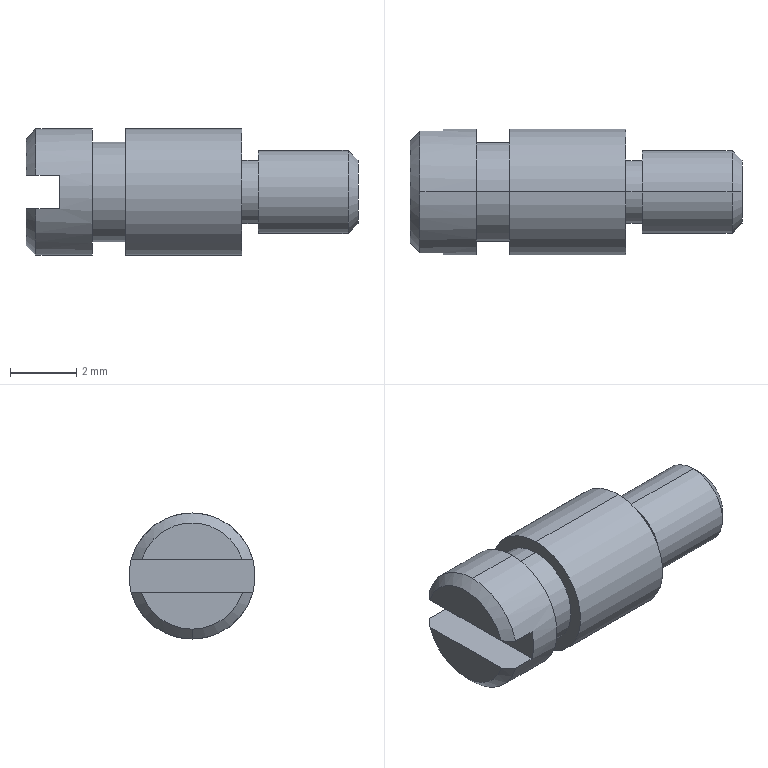Part | SolidWorks | features ICE 1, Revolution 1 | 1 solid | 25 faces | box 10 x 3.8 x 3.8 mm | volume 81.09 mm3 | cylinder 10 | plane 10 | cone 5 | commonest cylinder face diameters 3.8 x4 1.9 x2 2.5 x2 3 x2
STEP:
#1=CARTESIAN_POINT('',(0.,0.,0.95));
#2=VERTEX_POINT('',#1);
#3=CARTESIAN_POINT('',(0.,0.,-0.95));
#4=VERTEX_POINT('',#3);
#5=CARTESIAN_POINT('',(0.,0.,0.));
#6=DIRECTION('',(-1.,0.,0.));
#7=DIRECTION('',(0.,0.,1.));
#8=AXIS2_PLACEMENT_3D('',#5,#6,#7);
#9=CIRCLE('',#8,0.95);
#10=EDGE_CURVE('',#2,#4,#9,.T.);
#11=ORIENTED_EDGE('',*,*,#10,.T.);
#12=CARTESIAN_POINT('',(-0.3,0.,-1.25));
#13=VERTEX_POINT('',#12);
#14=CARTESIAN_POINT('',(0.,0.,-0.95));
#15=DIRECTION('',(-0.7071,0.,-0.7071));
#16=VECTOR('',#15,1000.);
#17=LINE('',#14,#16);
#18=EDGE_CURVE('',#4,#13,#17,.T.);
#19=ORIENTED_EDGE('',*,*,#18,.T.);
#20=CARTESIAN_POINT('',(-0.3,0.,1.25));
#21=VERTEX_POINT('',#20);
#22=CARTESIAN_POINT('',(-0.3,0.,0.));
#23=DIRECTION('',(-1.,0.,0.));
#24=DIRECTION('',(0.,0.,1.));
#25=AXIS2_PLACEMENT_3D('',#22,#23,#24);
#26=CIRCLE('',#25,1.25);
#27=EDGE_CURVE('',#21,#13,#26,.T.);
#28=ORIENTED_EDGE('',*,*,#27,.F.);
#29=CARTESIAN_POINT('',(0.,0.,0.95));
#30=DIRECTION('',(-0.7071,0.,0.7071));
#31=VECTOR('',#30,1000.);
#32=LINE('',#29,#31);
#33=EDGE_CURVE('',#2,#21,#32,.T.);
#34=ORIENTED_EDGE('',*,*,#33,.F.);
#35=EDGE_LOOP('',(#11,#19,#28,#34));
#36=FACE_OUTER_BOUND('',#35,.T.);
#37=CARTESIAN_POINT('',(0.,0.,0.));
#38=DIRECTION('',(-1.,0.,0.));
#39=DIRECTION('',(0.,0.,1.));
#40=AXIS2_PLACEMENT_3D('',#37,#38,#39);
#41=CONICAL_SURFACE('',#40,0.95,0.7854);
#42=ADVANCED_FACE('',(#36),#41,.T.);
#43=ORIENTED_EDGE('',*,*,#27,.T.);
#44=CARTESIAN_POINT('',(-3.,0.,-1.25));
#45=VERTEX_POINT('',#44);
#46=CARTESIAN_POINT('',(0.,0.,-1.25));
#47=DIRECTION('',(-1.,0.,0.));
#48=VECTOR('',#47,1000.);
#49=LINE('',#46,#48);
#50=EDGE_CURVE('',#13,#45,#49,.T.);
#51=ORIENTED_EDGE('',*,*,#50,.T.);
#52=CARTESIAN_POINT('',(-3.,0.,1.25));
#53=VERTEX_POINT('',#52);
#54=CARTESIAN_POINT('',(-3.,0.,0.));
#55=DIRECTION('',(-1.,0.,0.));
#56=DIRECTION('',(0.,0.,1.));
#57=AXIS2_PLACEMENT_3D('',#54,#55,#56);
#58=CIRCLE('',#57,1.25);
#59=EDGE_CURVE('',#53,#45,#58,.T.);
#60=ORIENTED_EDGE('',*,*,#59,.F.);
#61=CARTESIAN_POINT('',(0.,0.,1.25));
#62=DIRECTION('',(-1.,0.,0.));
#63=VECTOR('',#62,1000.);
#64=LINE('',#61,#63);
#65=EDGE_CURVE('',#21,#53,#64,.T.);
#66=ORIENTED_EDGE('',*,*,#65,.F.);
#67=EDGE_LOOP('',(#43,#51,#60,#66));
#68=FACE_OUTER_BOUND('',#67,.T.);
#69=CARTESIAN_POINT('',(0.,0.,0.));
#70=DIRECTION('',(-1.,0.,0.));
#71=DIRECTION('',(0.,0.,1.));
#72=AXIS2_PLACEMENT_3D('',#69,#70,#71);
#73=CYLINDRICAL_SURFACE('',#72,1.25);
#74=ADVANCED_FACE('',(#68),#73,.T.);
#75=CARTESIAN_POINT('',(-3.,0.,0.95));
#76=VERTEX_POINT('',#75);
#77=CARTESIAN_POINT('',(-3.,0.,-0.95));
#78=VERTEX_POINT('',#77);
#79=CARTESIAN_POINT('',(-3.,0.,0.));
#80=DIRECTION('',(-1.,0.,0.));
#81=DIRECTION('',(0.,0.,1.));
#82=AXIS2_PLACEMENT_3D('',#79,#80,#81);
#83=CIRCLE('',#82,0.95);
#84=EDGE_CURVE('',#76,#78,#83,.T.);
#85=ORIENTED_EDGE('',*,*,#84,.T.);
#86=CARTESIAN_POINT('',(-3.5,0.,-0.95));
#87=VERTEX_POINT('',#86);
#88=CARTESIAN_POINT('',(0.,0.,-0.95));
#89=DIRECTION('',(-1.,0.,0.));
#90=VECTOR('',#89,1000.);
#91=LINE('',#88,#90);
#92=EDGE_CURVE('',#78,#87,#91,.T.);
#93=ORIENTED_EDGE('',*,*,#92,.T.);
#94=CARTESIAN_POINT('',(-3.5,0.,0.95));
#95=VERTEX_POINT('',#94);
#96=CARTESIAN_POINT('',(-3.5,0.,0.));
#97=DIRECTION('',(-1.,0.,0.));
#98=DIRECTION('',(0.,0.,1.));
#99=AXIS2_PLACEMENT_3D('',#96,#97,#98);
#100=CIRCLE('',#99,0.95);
#101=EDGE_CURVE('',#95,#87,#100,.T.);
#102=ORIENTED_EDGE('',*,*,#101,.F.);
#103=CARTESIAN_POINT('',(0.,0.,0.95));
#104=DIRECTION('',(-1.,0.,0.));
#105=VECTOR('',#104,1000.);
#106=LINE('',#103,#105);
#107=EDGE_CURVE('',#76,#95,#106,.T.);
#108=ORIENTED_EDGE('',*,*,#107,.F.);
#109=EDGE_LOOP('',(#85,#93,#102,#108));
#110=FACE_OUTER_BOUND('',#109,.T.);
#111=CARTESIAN_POINT('',(0.,0.,0.));
#112=DIRECTION('',(-1.,0.,0.));
#113=DIRECTION('',(0.,0.,1.));
#114=AXIS2_PLACEMENT_3D('',#111,#112,#113);
#115=CYLINDRICAL_SURFACE('',#114,0.95);
#116=ADVANCED_FACE('',(#110),#115,.T.);
#117=CARTESIAN_POINT('',(-3.5,0.,1.9));
#118=VERTEX_POINT('',#117);
#119=CARTESIAN_POINT('',(-3.5,0.,-1.9));
#120=VERTEX_POINT('',#119);
#121=CARTESIAN_POINT('',(-3.5,0.,0.));
#122=DIRECTION('',(-1.,0.,0.));
#123=DIRECTION('',(0.,0.,1.));
#124=AXIS2_PLACEMENT_3D('',#121,#122,#123);
#125=CIRCLE('',#124,1.9);
#126=EDGE_CURVE('',#118,#120,#125,.T.);
#127=ORIENTED_EDGE('',*,*,#126,.T.);
#128=CARTESIAN_POINT('',(-7.,0.,-1.9));
#129=VERTEX_POINT('',#128);
#130=CARTESIAN_POINT('',(0.,0.,-1.9));
#131=DIRECTION('',(-1.,0.,0.));
#132=VECTOR('',#131,1000.);
#133=LINE('',#130,#132);
#134=EDGE_CURVE('',#120,#129,#133,.T.);
#135=ORIENTED_EDGE('',*,*,#134,.T.);
#136=CARTESIAN_POINT('',(-7.,0.,1.9));
#137=VERTEX_POINT('',#136);
#138=CARTESIAN_POINT('',(-7.,0.,0.));
#139=DIRECTION('',(-1.,0.,0.));
#140=DIRECTION('',(0.,0.,1.));
#141=AXIS2_PLACEMENT_3D('',#138,#139,#140);
#142=CIRCLE('',#141,1.9);
#143=EDGE_CURVE('',#137,#129,#142,.T.);
#144=ORIENTED_EDGE('',*,*,#143,.F.);
#145=CARTESIAN_POINT('',(0.,0.,1.9));
#146=DIRECTION('',(-1.,0.,0.));
#147=VECTOR('',#146,1000.);
#148=LINE('',#145,#147);
#149=EDGE_CURVE('',#118,#137,#148,.T.);
#150=ORIENTED_EDGE('',*,*,#149,.F.);
#151=EDGE_LOOP('',(#127,#135,#144,#150));
#152=FACE_OUTER_BOUND('',#151,.T.);
#153=CARTESIAN_POINT('',(0.,0.,0.));
#154=DIRECTION('',(-1.,0.,0.));
#155=DIRECTION('',(0.,0.,1.));
#156=AXIS2_PLACEMENT_3D('',#153,#154,#155);
#157=CYLINDRICAL_SURFACE('',#156,1.9);
#158=ADVANCED_FACE('',(#152),#157,.T.);
#159=CARTESIAN_POINT('',(-7.,0.,1.5));
#160=VERTEX_POINT('',#159);
#161=CARTESIAN_POINT('',(-7.,0.,-1.5));
#162=VERTEX_POINT('',#161);
#163=CARTESIAN_POINT('',(-7.,0.,0.));
#164=DIRECTION('',(-1.,0.,0.));
#165=DIRECTION('',(0.,0.,1.));
#166=AXIS2_PLACEMENT_3D('',#163,#164,#165);
#167=CIRCLE('',#166,1.5);
#168=EDGE_CURVE('',#160,#162,#167,.T.);
#169=ORIENTED_EDGE('',*,*,#168,.T.);
#170=CARTESIAN_POINT('',(-8.,0.,-1.5));
#171=VERTEX_POINT('',#170);
#172=CARTESIAN_POINT('',(0.,0.,-1.5));
#173=DIRECTION('',(-1.,0.,0.));
#174=VECTOR('',#173,1000.);
#175=LINE('',#172,#174);
#176=EDGE_CURVE('',#162,#171,#175,.T.);
#177=ORIENTED_EDGE('',*,*,#176,.T.);
#178=CARTESIAN_POINT('',(-8.,0.,1.5));
#179=VERTEX_POINT('',#178);
#180=CARTESIAN_POINT('',(-8.,0.,0.));
#181=DIRECTION('',(-1.,0.,0.));
#182=DIRECTION('',(0.,0.,1.));
#183=AXIS2_PLACEMENT_3D('',#180,#181,#182);
#184=CIRCLE('',#183,1.5);
#185=EDGE_CURVE('',#179,#171,#184,.T.);
#186=ORIENTED_EDGE('',*,*,#185,.F.);
#187=CARTESIAN_POINT('',(0.,0.,1.5));
#188=DIRECTION('',(-1.,0.,0.));
#189=VECTOR('',#188,1000.);
#190=LINE('',#187,#189);
#191=EDGE_CURVE('',#160,#179,#190,.T.);
#192=ORIENTED_EDGE('',*,*,#191,.F.);
#193=EDGE_LOOP('',(#169,#177,#186,#192));
#194=FACE_OUTER_BOUND('',#193,.T.);
#195=CARTESIAN_POINT('',(0.,0.,0.));
#196=DIRECTION('',(-1.,0.,0.));
#197=DIRECTION('',(0.,0.,1.));
#198=AXIS2_PLACEMENT_3D('',#195,#196,#197);
#199=CYLINDRICAL_SURFACE('',#198,1.5);
#200=ADVANCED_FACE('',(#194),#199,.T.);
#201=CARTESIAN_POINT('',(-8.,0.,1.9));
#202=VERTEX_POINT('',#201);
#203=CARTESIAN_POINT('',(-8.,0.,-1.9));
#204=VERTEX_POINT('',#203);
#205=CARTESIAN_POINT('',(-8.,0.,0.));
#206=DIRECTION('',(-1.,0.,0.));
#207=DIRECTION('',(0.,0.,1.));
#208=AXIS2_PLACEMENT_3D('',#205,#206,#207);
#209=CIRCLE('',#208,1.9);
#210=EDGE_CURVE('',#202,#204,#209,.T.);
#211=ORIENTED_EDGE('',*,*,#210,.T.);
#212=CARTESIAN_POINT('',(-9.7,0.,-1.9));
#213=VERTEX_POINT('',#212);
#214=CARTESIAN_POINT('',(0.,0.,-1.9));
#215=DIRECTION('',(-1.,0.,0.));
#216=VECTOR('',#215,1000.);
#217=LINE('',#214,#216);
#218=EDGE_CURVE('',#204,#213,#217,.T.);
#219=ORIENTED_EDGE('',*,*,#218,.T.);
#220=CARTESIAN_POINT('',(-9.7,1.833,-0.5));
#221=VERTEX_POINT('',#220);
#222=CARTESIAN_POINT('',(-9.7,0.,0.));
#223=DIRECTION('',(-1.,0.,0.));
#224=DIRECTION('',(0.,0.,1.));
#225=AXIS2_PLACEMENT_3D('',#222,#223,#224);
#226=CIRCLE('',#225,1.9);
#227=EDGE_CURVE('',#221,#213,#226,.T.);
#228=ORIENTED_EDGE('',*,*,#227,.F.);
#229=CARTESIAN_POINT('',(-9.,1.833,-0.5));
#230=VERTEX_POINT('',#229);
#231=CARTESIAN_POINT('',(0.,1.833,-0.5));
#232=DIRECTION('',(1.,0.,0.));
#233=VECTOR('',#232,1000.);
#234=LINE('',#231,#233);
#235=EDGE_CURVE('',#221,#230,#234,.T.);
#236=ORIENTED_EDGE('',*,*,#235,.T.);
#237=CARTESIAN_POINT('',(-9.,1.833,0.5));
#238=VERTEX_POINT('',#237);
#239=CARTESIAN_POINT('',(-9.,0.,0.));
#240=DIRECTION('',(-1.,0.,0.));
#241=DIRECTION('',(0.,0.,1.));
#242=AXIS2_PLACEMENT_3D('',#239,#240,#241);
#243=CIRCLE('',#242,1.9);
#244=EDGE_CURVE('',#238,#230,#243,.T.);
#245=ORIENTED_EDGE('',*,*,#244,.F.);
#246=CARTESIAN_POINT('',(-9.7,1.833,0.5));
#247=VERTEX_POINT('',#246);
#248=CARTESIAN_POINT('',(0.,1.833,0.5));
#249=DIRECTION('',(-1.,0.,0.));
#250=VECTOR('',#249,1000.);
#251=LINE('',#248,#250);
#252=EDGE_CURVE('',#238,#247,#251,.T.);
#253=ORIENTED_EDGE('',*,*,#252,.T.);
#254=CARTESIAN_POINT('',(-9.7,0.,1.9));
#255=VERTEX_POINT('',#254);
#256=CARTESIAN_POINT('',(-9.7,0.,0.));
#257=DIRECTION('',(-1.,0.,0.));
#258=DIRECTION('',(0.,0.,1.));
#259=AXIS2_PLACEMENT_3D('',#256,#257,#258);
#260=CIRCLE('',#259,1.9);
#261=EDGE_CURVE('',#255,#247,#260,.T.);
#262=ORIENTED_EDGE('',*,*,#261,.F.);
#263=CARTESIAN_POINT('',(0.,0.,1.9));
#264=DIRECTION('',(-1.,0.,0.));
#265=VECTOR('',#264,1000.);
#266=LINE('',#263,#265);
#267=EDGE_CURVE('',#202,#255,#266,.T.);
#268=ORIENTED_EDGE('',*,*,#267,.F.);
#269=EDGE_LOOP('',(#211,#219,#228,#236,#245,#253,#262,#268));
#270=FACE_OUTER_BOUND('',#269,.T.);
#271=CARTESIAN_POINT('',(0.,0.,0.));
#272=DIRECTION('',(-1.,0.,0.));
#273=DIRECTION('',(0.,0.,1.));
#274=AXIS2_PLACEMENT_3D('',#271,#272,#273);
#275=CYLINDRICAL_SURFACE('',#274,1.9);
#276=ADVANCED_FACE('',(#270),#275,.T.);
#277=CARTESIAN_POINT('',(-10.,0.,-1.6));
#278=VERTEX_POINT('',#277);
#279=CARTESIAN_POINT('',(-10.,-1.52,-0.5));
#280=VERTEX_POINT('',#279);
#281=CARTESIAN_POINT('',(-10.,0.,0.));
#282=DIRECTION('',(-1.,0.,0.));
#283=DIRECTION('',(0.,0.,1.));
#284=AXIS2_PLACEMENT_3D('',#281,#282,#283);
#285=CIRCLE('',#284,1.6);
#286=EDGE_CURVE('',#278,#280,#285,.T.);
#287=ORIENTED_EDGE('',*,*,#286,.F.);
#288=CARTESIAN_POINT('',(-9.7,0.,-1.9));
#289=DIRECTION('',(0.7071,0.,-0.7071));
#290=VECTOR('',#289,1000.);
#291=LINE('',#288,#290);
#292=EDGE_CURVE('',#278,#213,#291,.T.);
#293=ORIENTED_EDGE('',*,*,#292,.T.);
#294=CARTESIAN_POINT('',(-9.7,-1.833,-0.5));
#295=VERTEX_POINT('',#294);
#296=CARTESIAN_POINT('',(-9.7,0.,0.));
#297=DIRECTION('',(-1.,0.,0.));
#298=DIRECTION('',(0.,0.,1.));
#299=AXIS2_PLACEMENT_3D('',#296,#297,#298);
#300=CIRCLE('',#299,1.9);
#301=EDGE_CURVE('',#213,#295,#300,.T.);
#302=ORIENTED_EDGE('',*,*,#301,.T.);
#303=CARTESIAN_POINT('',(-9.7,-1.833,-0.5));
#304=CARTESIAN_POINT('',(-9.8,-1.729,-0.5));
#305=CARTESIAN_POINT('',(-9.9,-1.625,-0.5));
#306=CARTESIAN_POINT('',(-10.,-1.52,-0.5));
#307=B_SPLINE_CURVE_WITH_KNOTS('',3,(#303,#304,#305,#306),.UNSPECIFIED.,.F.,.F.,(4,4),(0.003261,0.003694),.UNSPECIFIED.);
#308=EDGE_CURVE('',#295,#280,#307,.T.);
#309=ORIENTED_EDGE('',*,*,#308,.T.);
#310=EDGE_LOOP('',(#287,#293,#302,#309));
#311=FACE_OUTER_BOUND('',#310,.T.);
#312=CARTESIAN_POINT('',(-9.7,0.,0.));
#313=DIRECTION('',(1.,0.,0.));
#314=DIRECTION('',(0.,0.,-1.));
#315=AXIS2_PLACEMENT_3D('',#312,#313,#314);
#316=CONICAL_SURFACE('',#315,1.9,0.7854);
#317=ADVANCED_FACE('',(#311),#316,.T.);
#318=CARTESIAN_POINT('',(-10.,-1.52,0.5));
#319=VERTEX_POINT('',#318);
#320=CARTESIAN_POINT('',(-10.,1.52,0.5));
#321=VERTEX_POINT('',#320);
#322=CARTESIAN_POINT('',(-10.,0.,0.));
#323=DIRECTION('',(-1.,0.,0.));
#324=DIRECTION('',(0.,0.,1.));
#325=AXIS2_PLACEMENT_3D('',#322,#323,#324);
#326=CIRCLE('',#325,1.6);
#327=EDGE_CURVE('',#319,#321,#326,.T.);
#328=ORIENTED_EDGE('',*,*,#327,.T.);
#329=CARTESIAN_POINT('',(-10.,3.388,0.5));
#330=DIRECTION('',(0.,1.,0.));
#331=VECTOR('',#330,1000.);
#332=LINE('',#329,#331);
#333=EDGE_CURVE('',#319,#321,#332,.T.);
#334=ORIENTED_EDGE('',*,*,#333,.F.);
#335=EDGE_LOOP('',(#328,#334));
#336=FACE_OUTER_BOUND('',#335,.T.);
#337=CARTESIAN_POINT('',(-10.,0.,0.));
#338=DIRECTION('',(1.,0.,0.));
#339=DIRECTION('',(0.,0.,-1.));
#340=AXIS2_PLACEMENT_3D('',#337,#338,#339);
#341=PLANE('',#340);
#342=ADVANCED_FACE('',(#336),#341,.F.);
#343=CARTESIAN_POINT('',(-9.7,-1.833,0.5));
#344=VERTEX_POINT('',#343);
#345=CARTESIAN_POINT('',(-9.7,0.,0.));
#346=DIRECTION('',(-1.,0.,0.));
#347=DIRECTION('',(0.,0.,1.));
#348=AXIS2_PLACEMENT_3D('',#345,#346,#347);
#349=CIRCLE('',#348,1.9);
#350=EDGE_CURVE('',#344,#255,#349,.T.);
#351=ORIENTED_EDGE('',*,*,#350,.T.);
#352=ORIENTED_EDGE('',*,*,#261,.T.);
#353=CARTESIAN_POINT('',(-9.7,1.833,0.5));
#354=CARTESIAN_POINT('',(-9.8,1.729,0.5));
#355=CARTESIAN_POINT('',(-9.9,1.625,0.5));
#356=CARTESIAN_POINT('',(-10.,1.52,0.5));
#357=B_SPLINE_CURVE_WITH_KNOTS('',3,(#353,#354,#355,#356),.UNSPECIFIED.,.F.,.F.,(4,4),(0.003261,0.003694),.UNSPECIFIED.);
#358=EDGE_CURVE('',#247,#321,#357,.T.);
#359=ORIENTED_EDGE('',*,*,#358,.T.);
#360=ORIENTED_EDGE('',*,*,#327,.F.);
#361=CARTESIAN_POINT('',(-10.,-1.52,0.5));
#362=CARTESIAN_POINT('',(-9.9,-1.625,0.5));
#363=CARTESIAN_POINT('',(-9.8,-1.729,0.5));
#364=CARTESIAN_POINT('',(-9.7,-1.833,0.5));
#365=B_SPLINE_CURVE_WITH_KNOTS('',3,(#361,#362,#363,#364),.UNSPECIFIED.,.F.,.F.,(4,4),(0.007499,0.007933),.UNSPECIFIED.);
#366=EDGE_CURVE('',#319,#344,#365,.T.);
#367=ORIENTED_EDGE('',*,*,#366,.T.);
#368=EDGE_LOOP('',(#351,#352,#359,#360,#367));
#369=FACE_OUTER_BOUND('',#368,.T.);
#370=CARTESIAN_POINT('',(-9.7,0.,0.));
#371=DIRECTION('',(1.,0.,0.));
#372=DIRECTION('',(0.,0.,-1.));
#373=AXIS2_PLACEMENT_3D('',#370,#371,#372);
#374=CONICAL_SURFACE('',#373,1.9,0.7854);
#375=ADVANCED_FACE('',(#369),#374,.T.);
#376=ORIENTED_EDGE('',*,*,#10,.F.);
#377=CARTESIAN_POINT('',(0.,0.,0.));
#378=DIRECTION('',(-1.,0.,0.));
#379=DIRECTION('',(0.,0.,1.));
#380=AXIS2_PLACEMENT_3D('',#377,#378,#379);
#381=CIRCLE('',#380,0.95);
#382=EDGE_CURVE('',#4,#2,#381,.T.);
#383=ORIENTED_EDGE('',*,*,#382,.F.);
#384=EDGE_LOOP('',(#376,#383));
#385=FACE_OUTER_BOUND('',#384,.T.);
#386=CARTESIAN_POINT('',(0.,0.,-0.95));
#387=DIRECTION('',(-1.,0.,0.));
#388=DIRECTION('',(0.,0.,1.));
#389=AXIS2_PLACEMENT_3D('',#386,#387,#388);
#390=PLANE('',#389);
#391=ADVANCED_FACE('',(#385),#390,.F.);
#392=CARTESIAN_POINT('',(-10.,1.52,-0.5));
#393=VERTEX_POINT('',#392);
#394=CARTESIAN_POINT('',(-10.,0.,0.));
#395=DIRECTION('',(-1.,0.,0.));
#396=DIRECTION('',(0.,0.,1.));
#397=AXIS2_PLACEMENT_3D('',#394,#395,#396);
#398=CIRCLE('',#397,1.6);
#399=EDGE_CURVE('',#393,#278,#398,.T.);
#400=ORIENTED_EDGE('',*,*,#399,.T.);
#401=ORIENTED_EDGE('',*,*,#286,.T.);
#402=CARTESIAN_POINT('',(-10.,3.388,-0.5));
#403=DIRECTION('',(0.,-1.,0.));
#404=VECTOR('',#403,1000.);
#405=LINE('',#402,#404);
#406=EDGE_CURVE('',#393,#280,#405,.T.);
#407=ORIENTED_EDGE('',*,*,#406,.F.);
#408=EDGE_LOOP('',(#400,#401,#407));
#409=FACE_OUTER_BOUND('',#408,.T.);
#410=CARTESIAN_POINT('',(-10.,0.,0.));
#411=DIRECTION('',(1.,0.,0.));
#412=DIRECTION('',(0.,0.,-1.));
#413=AXIS2_PLACEMENT_3D('',#410,#411,#412);
#414=PLANE('',#413);
#415=ADVANCED_FACE('',(#409),#414,.F.);
#416=ORIENTED_EDGE('',*,*,#292,.F.);
#417=ORIENTED_EDGE('',*,*,#399,.F.);
#418=CARTESIAN_POINT('',(-10.,1.52,-0.5));
#419=CARTESIAN_POINT('',(-9.9,1.625,-0.5));
#420=CARTESIAN_POINT('',(-9.8,1.729,-0.5));
#421=CARTESIAN_POINT('',(-9.7,1.833,-0.5));
#422=B_SPLINE_CURVE_WITH_KNOTS('',3,(#418,#419,#420,#421),.UNSPECIFIED.,.F.,.F.,(4,4),(0.007499,0.007933),.UNSPECIFIED.);
#423=EDGE_CURVE('',#393,#221,#422,.T.);
#424=ORIENTED_EDGE('',*,*,#423,.T.);
#425=ORIENTED_EDGE('',*,*,#227,.T.);
#426=EDGE_LOOP('',(#416,#417,#424,#425));
#427=FACE_OUTER_BOUND('',#426,.T.);
#428=CARTESIAN_POINT('',(-9.7,0.,0.));
#429=DIRECTION('',(1.,0.,0.));
#430=DIRECTION('',(0.,0.,-1.));
#431=AXIS2_PLACEMENT_3D('',#428,#429,#430);
#432=CONICAL_SURFACE('',#431,1.9,0.7854);
#433=ADVANCED_FACE('',(#427),#432,.T.);
#434=ORIENTED_EDGE('',*,*,#218,.F.);
#435=CARTESIAN_POINT('',(-8.,0.,0.));
#436=DIRECTION('',(-1.,0.,0.));
#437=DIRECTION('',(0.,0.,1.));
#438=AXIS2_PLACEMENT_3D('',#435,#436,#437);
#439=CIRCLE('',#438,1.9);
#440=EDGE_CURVE('',#204,#202,#439,.T.);
#441=ORIENTED_EDGE('',*,*,#440,.T.);
#442=ORIENTED_EDGE('',*,*,#267,.T.);
#443=ORIENTED_EDGE('',*,*,#350,.F.);
#444=CARTESIAN_POINT('',(-9.,-1.833,0.5));
#445=VERTEX_POINT('',#444);
#446=CARTESIAN_POINT('',(0.,-1.833,0.5));
#447=DIRECTION('',(1.,0.,0.));
#448=VECTOR('',#447,1000.);
#449=LINE('',#446,#448);
#450=EDGE_CURVE('',#344,#445,#449,.T.);
#451=ORIENTED_EDGE('',*,*,#450,.T.);
#452=CARTESIAN_POINT('',(-9.,-1.833,-0.5));
#453=VERTEX_POINT('',#452);
#454=CARTESIAN_POINT('',(-9.,0.,0.));
#455=DIRECTION('',(-1.,0.,0.));
#456=DIRECTION('',(0.,0.,1.));
#457=AXIS2_PLACEMENT_3D('',#454,#455,#456);
#458=CIRCLE('',#457,1.9);
#459=EDGE_CURVE('',#453,#445,#458,.T.);
#460=ORIENTED_EDGE('',*,*,#459,.F.);
#461=CARTESIAN_POINT('',(0.,-1.833,-0.5));
#462=DIRECTION('',(-1.,0.,0.));
#463=VECTOR('',#462,1000.);
#464=LINE('',#461,#463);
#465=EDGE_CURVE('',#453,#295,#464,.T.);
#466=ORIENTED_EDGE('',*,*,#465,.T.);
#467=ORIENTED_EDGE('',*,*,#301,.F.);
#468=EDGE_LOOP('',(#434,#441,#442,#443,#451,#460,#466,#467));
#469=FACE_OUTER_BOUND('',#468,.T.);
#470=CARTESIAN_POINT('',(0.,0.,0.));
#471=DIRECTION('',(-1.,0.,0.));
#472=DIRECTION('',(0.,0.,1.));
#473=AXIS2_PLACEMENT_3D('',#470,#471,#472);
#474=CYLINDRICAL_SURFACE('',#473,1.9);
#475=ADVANCED_FACE('',(#469),#474,.T.);
#476=ORIENTED_EDGE('',*,*,#210,.F.);
#477=ORIENTED_EDGE('',*,*,#440,.F.);
#478=EDGE_LOOP('',(#476,#477));
#479=FACE_OUTER_BOUND('',#478,.T.);
#480=ORIENTED_EDGE('',*,*,#185,.T.);
#481=CARTESIAN_POINT('',(-8.,0.,0.));
#482=DIRECTION('',(-1.,0.,0.));
#483=DIRECTION('',(0.,0.,1.));
#484=AXIS2_PLACEMENT_3D('',#481,#482,#483);
#485=CIRCLE('',#484,1.5);
#486=EDGE_CURVE('',#171,#179,#485,.T.);
#487=ORIENTED_EDGE('',*,*,#486,.T.);
#488=EDGE_LOOP('',(#480,#487));
#489=FACE_BOUND('',#488,.T.);
#490=CARTESIAN_POINT('',(-8.,0.,-1.9));
#491=DIRECTION('',(-1.,0.,0.));
#492=DIRECTION('',(0.,0.,1.));
#493=AXIS2_PLACEMENT_3D('',#490,#491,#492);
#494=PLANE('',#493);
#495=ADVANCED_FACE('',(#479,#489),#494,.F.);
#496=ORIENTED_EDGE('',*,*,#176,.F.);
#497=CARTESIAN_POINT('',(-7.,0.,0.));
#498=DIRECTION('',(-1.,0.,0.));
#499=DIRECTION('',(0.,0.,1.));
#500=AXIS2_PLACEMENT_3D('',#497,#498,#499);
#501=CIRCLE('',#500,1.5);
#502=EDGE_CURVE('',#162,#160,#501,.T.);
#503=ORIENTED_EDGE('',*,*,#502,.T.);
#504=ORIENTED_EDGE('',*,*,#191,.T.);
#505=ORIENTED_EDGE('',*,*,#486,.F.);
#506=EDGE_LOOP('',(#496,#503,#504,#505));
#507=FACE_OUTER_BOUND('',#506,.T.);
#508=CARTESIAN_POINT('',(0.,0.,0.));
#509=DIRECTION('',(-1.,0.,0.));
#510=DIRECTION('',(0.,0.,1.));
#511=AXIS2_PLACEMENT_3D('',#508,#509,#510);
#512=CYLINDRICAL_SURFACE('',#511,1.5);
#513=ADVANCED_FACE('',(#507),#512,.T.);
#514=ORIENTED_EDGE('',*,*,#168,.F.);
#515=ORIENTED_EDGE('',*,*,#502,.F.);
#516=EDGE_LOOP('',(#514,#515));
#517=FACE_BOUND('',#516,.T.);
#518=ORIENTED_EDGE('',*,*,#143,.T.);
#519=CARTESIAN_POINT('',(-7.,0.,0.));
#520=DIRECTION('',(-1.,0.,0.));
#521=DIRECTION('',(0.,0.,1.));
#522=AXIS2_PLACEMENT_3D('',#519,#520,#521);
#523=CIRCLE('',#522,1.9);
#524=EDGE_CURVE('',#129,#137,#523,.T.);
#525=ORIENTED_EDGE('',*,*,#524,.T.);
#526=EDGE_LOOP('',(#518,#525));
#527=FACE_OUTER_BOUND('',#526,.T.);
#528=CARTESIAN_POINT('',(-7.,0.,-1.5));
#529=DIRECTION('',(1.,0.,0.));
#530=DIRECTION('',(0.,0.,-1.));
#531=AXIS2_PLACEMENT_3D('',#528,#529,#530);
#532=PLANE('',#531);
#533=ADVANCED_FACE('',(#517,#527),#532,.F.);
#534=ORIENTED_EDGE('',*,*,#134,.F.);
#535=CARTESIAN_POINT('',(-3.5,0.,0.));
#536=DIRECTION('',(-1.,0.,0.));
#537=DIRECTION('',(0.,0.,1.));
#538=AXIS2_PLACEMENT_3D('',#535,#536,#537);
#539=CIRCLE('',#538,1.9);
#540=EDGE_CURVE('',#120,#118,#539,.T.);
#541=ORIENTED_EDGE('',*,*,#540,.T.);
#542=ORIENTED_EDGE('',*,*,#149,.T.);
#543=ORIENTED_EDGE('',*,*,#524,.F.);
#544=EDGE_LOOP('',(#534,#541,#542,#543));
#545=FACE_OUTER_BOUND('',#544,.T.);
#546=CARTESIAN_POINT('',(0.,0.,0.));
#547=DIRECTION('',(-1.,0.,0.));
#548=DIRECTION('',(0.,0.,1.));
#549=AXIS2_PLACEMENT_3D('',#546,#547,#548);
#550=CYLINDRICAL_SURFACE('',#549,1.9);
#551=ADVANCED_FACE('',(#545),#550,.T.);
#552=ORIENTED_EDGE('',*,*,#126,.F.);
#553=ORIENTED_EDGE('',*,*,#540,.F.);
#554=EDGE_LOOP('',(#552,#553));
#555=FACE_OUTER_BOUND('',#554,.T.);
#556=ORIENTED_EDGE('',*,*,#101,.T.);
#557=CARTESIAN_POINT('',(-3.5,0.,0.));
#558=DIRECTION('',(-1.,0.,0.));
#559=DIRECTION('',(0.,0.,1.));
#560=AXIS2_PLACEMENT_3D('',#557,#558,#559);
#561=CIRCLE('',#560,0.95);
#562=EDGE_CURVE('',#87,#95,#561,.T.);
#563=ORIENTED_EDGE('',*,*,#562,.T.);
#564=EDGE_LOOP('',(#556,#563));
#565=FACE_BOUND('',#564,.T.);
#566=CARTESIAN_POINT('',(-3.5,0.,-1.9));
#567=DIRECTION('',(-1.,0.,0.));
#568=DIRECTION('',(0.,0.,1.));
#569=AXIS2_PLACEMENT_3D('',#566,#567,#568);
#570=PLANE('',#569);
#571=ADVANCED_FACE('',(#555,#565),#570,.F.);
#572=ORIENTED_EDGE('',*,*,#92,.F.);
#573=CARTESIAN_POINT('',(-3.,0.,0.));
#574=DIRECTION('',(-1.,0.,0.));
#575=DIRECTION('',(0.,0.,1.));
#576=AXIS2_PLACEMENT_3D('',#573,#574,#575);
#577=CIRCLE('',#576,0.95);
#578=EDGE_CURVE('',#78,#76,#577,.T.);
#579=ORIENTED_EDGE('',*,*,#578,.T.);
#580=ORIENTED_EDGE('',*,*,#107,.T.);
#581=ORIENTED_EDGE('',*,*,#562,.F.);
#582=EDGE_LOOP('',(#572,#579,#580,#581));
#583=FACE_OUTER_BOUND('',#582,.T.);
#584=CARTESIAN_POINT('',(0.,0.,0.));
#585=DIRECTION('',(-1.,0.,0.));
#586=DIRECTION('',(0.,0.,1.));
#587=AXIS2_PLACEMENT_3D('',#584,#585,#586);
#588=CYLINDRICAL_SURFACE('',#587,0.95);
#589=ADVANCED_FACE('',(#583),#588,.T.);
#590=ORIENTED_EDGE('',*,*,#84,.F.);
#591=ORIENTED_EDGE('',*,*,#578,.F.);
#592=EDGE_LOOP('',(#590,#591));
#593=FACE_BOUND('',#592,.T.);
#594=ORIENTED_EDGE('',*,*,#59,.T.);
#595=CARTESIAN_POINT('',(-3.,0.,0.));
#596=DIRECTION('',(-1.,0.,0.));
#597=DIRECTION('',(0.,0.,1.));
#598=AXIS2_PLACEMENT_3D('',#595,#596,#597);
#599=CIRCLE('',#598,1.25);
#600=EDGE_CURVE('',#45,#53,#599,.T.);
#601=ORIENTED_EDGE('',*,*,#600,.T.);
#602=EDGE_LOOP('',(#594,#601));
#603=FACE_OUTER_BOUND('',#602,.T.);
#604=CARTESIAN_POINT('',(-3.,0.,-1.25));
#605=DIRECTION('',(1.,0.,0.));
#606=DIRECTION('',(0.,0.,-1.));
#607=AXIS2_PLACEMENT_3D('',#604,#605,#606);
#608=PLANE('',#607);
#609=ADVANCED_FACE('',(#593,#603),#608,.F.);
#610=ORIENTED_EDGE('',*,*,#50,.F.);
#611=CARTESIAN_POINT('',(-0.3,0.,0.));
#612=DIRECTION('',(-1.,0.,0.));
#613=DIRECTION('',(0.,0.,1.));
#614=AXIS2_PLACEMENT_3D('',#611,#612,#613);
#615=CIRCLE('',#614,1.25);
#616=EDGE_CURVE('',#13,#21,#615,.T.);
#617=ORIENTED_EDGE('',*,*,#616,.T.);
#618=ORIENTED_EDGE('',*,*,#65,.T.);
#619=ORIENTED_EDGE('',*,*,#600,.F.);
#620=EDGE_LOOP('',(#610,#617,#618,#619));
#621=FACE_OUTER_BOUND('',#620,.T.);
#622=CARTESIAN_POINT('',(0.,0.,0.));
#623=DIRECTION('',(-1.,0.,0.));
#624=DIRECTION('',(0.,0.,1.));
#625=AXIS2_PLACEMENT_3D('',#622,#623,#624);
#626=CYLINDRICAL_SURFACE('',#625,1.25);
#627=ADVANCED_FACE('',(#621),#626,.T.);
#628=ORIENTED_EDGE('',*,*,#18,.F.);
#629=ORIENTED_EDGE('',*,*,#382,.T.);
#630=ORIENTED_EDGE('',*,*,#33,.T.);
#631=ORIENTED_EDGE('',*,*,#616,.F.);
#632=EDGE_LOOP('',(#628,#629,#630,#631));
#633=FACE_OUTER_BOUND('',#632,.T.);
#634=CARTESIAN_POINT('',(0.,0.,0.));
#635=DIRECTION('',(-1.,0.,0.));
#636=DIRECTION('',(0.,0.,1.));
#637=AXIS2_PLACEMENT_3D('',#634,#635,#636);
#638=CONICAL_SURFACE('',#637,0.95,0.7854);
#639=ADVANCED_FACE('',(#633),#638,.T.);
#640=ORIENTED_EDGE('',*,*,#252,.F.);
#641=CARTESIAN_POINT('',(-9.,3.388,0.5));
#642=DIRECTION('',(0.,1.,0.));
#643=VECTOR('',#642,1000.);
#644=LINE('',#641,#643);
#645=EDGE_CURVE('',#445,#238,#644,.T.);
#646=ORIENTED_EDGE('',*,*,#645,.F.);
#647=ORIENTED_EDGE('',*,*,#450,.F.);
#648=ORIENTED_EDGE('',*,*,#366,.F.);
#649=ORIENTED_EDGE('',*,*,#333,.T.);
#650=ORIENTED_EDGE('',*,*,#358,.F.);
#651=EDGE_LOOP('',(#640,#646,#647,#648,#649,#650));
#652=FACE_OUTER_BOUND('',#651,.T.);
#653=CARTESIAN_POINT('',(-9.,3.388,0.5));
#654=DIRECTION('',(0.,0.,1.));
#655=DIRECTION('',(0.,-1.,0.));
#656=AXIS2_PLACEMENT_3D('',#653,#654,#655);
#657=PLANE('',#656);
#658=ADVANCED_FACE('',(#652),#657,.F.);
#659=ORIENTED_EDGE('',*,*,#465,.F.);
#660=CARTESIAN_POINT('',(-9.,3.388,-0.5));
#661=DIRECTION('',(0.,-1.,0.));
#662=VECTOR('',#661,1000.);
#663=LINE('',#660,#662);
#664=EDGE_CURVE('',#230,#453,#663,.T.);
#665=ORIENTED_EDGE('',*,*,#664,.F.);
#666=ORIENTED_EDGE('',*,*,#235,.F.);
#667=ORIENTED_EDGE('',*,*,#423,.F.);
#668=ORIENTED_EDGE('',*,*,#406,.T.);
#669=ORIENTED_EDGE('',*,*,#308,.F.);
#670=EDGE_LOOP('',(#659,#665,#666,#667,#668,#669));
#671=FACE_OUTER_BOUND('',#670,.T.);
#672=CARTESIAN_POINT('',(-9.,3.388,-0.5));
#673=DIRECTION('',(0.,0.,-1.));
#674=DIRECTION('',(0.,1.,0.));
#675=AXIS2_PLACEMENT_3D('',#672,#673,#674);
#676=PLANE('',#675);
#677=ADVANCED_FACE('',(#671),#676,.F.);
#678=ORIENTED_EDGE('',*,*,#244,.T.);
#679=ORIENTED_EDGE('',*,*,#664,.T.);
#680=ORIENTED_EDGE('',*,*,#459,.T.);
#681=ORIENTED_EDGE('',*,*,#645,.T.);
#682=EDGE_LOOP('',(#678,#679,#680,#681));
#683=FACE_OUTER_BOUND('',#682,.T.);
#684=CARTESIAN_POINT('',(-9.,0.,0.));
#685=DIRECTION('',(-1.,0.,0.));
#686=DIRECTION('',(0.,0.,1.));
#687=AXIS2_PLACEMENT_3D('',#684,#685,#686);
#688=PLANE('',#687);
#689=ADVANCED_FACE('',(#683),#688,.T.);
#690=CLOSED_SHELL('',(#42,#74,#116,#158,#200,#276,#317,#342,#375,#391,#415,#433,#475,#495,#513,#533,#551,#571,#589,#609,#627,#639,#658,#677,#689));
#691=MANIFOLD_SOLID_BREP('',#690);
#692=CARTESIAN_POINT('',(0.,0.,0.));
#693=DIRECTION('',(0.,0.,1.));
#694=DIRECTION('',(1.,0.,0.));
#695=AXIS2_PLACEMENT_3D('',#692,#693,#694);
#696=(LENGTH_UNIT()NAMED_UNIT(*)SI_UNIT(.MILLI.,.METRE.));
#697=UNCERTAINTY_MEASURE_WITH_UNIT(LENGTH_MEASURE(0.00001),#696,'','');
#698=(NAMED_UNIT(*)PLANE_ANGLE_UNIT()SI_UNIT($,.RADIAN.));
#699=(NAMED_UNIT(*)SI_UNIT($,.STERADIAN.)SOLID_ANGLE_UNIT());
#700=(GEOMETRIC_REPRESENTATION_CONTEXT(3)GLOBAL_UNCERTAINTY_ASSIGNED_CONTEXT((#697))GLOBAL_UNIT_ASSIGNED_CONTEXT((#696,#698,#699))REPRESENTATION_CONTEXT('',''));
#701=ADVANCED_BREP_SHAPE_REPRESENTATION('',(#691,#695),#700);